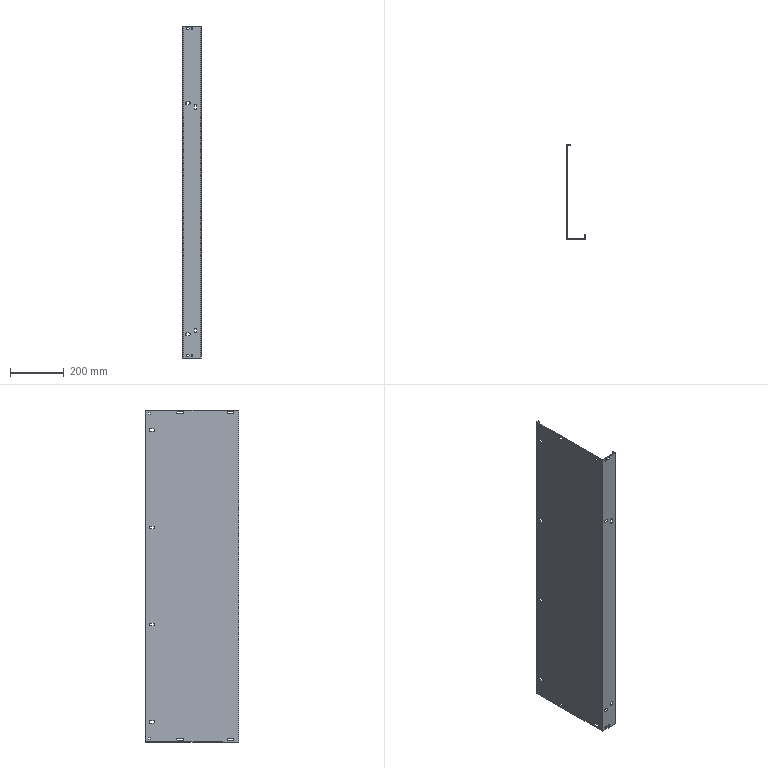Part | 1 solid | 132 faces | box 70 x 349.5 x 1240 mm | volume 821379 mm3 | plane 88 | cylinder 44 | commonest cylinder face diameters 9 x12 10 x12 11 x10 8 x4 0.4 x3 3.4 x3